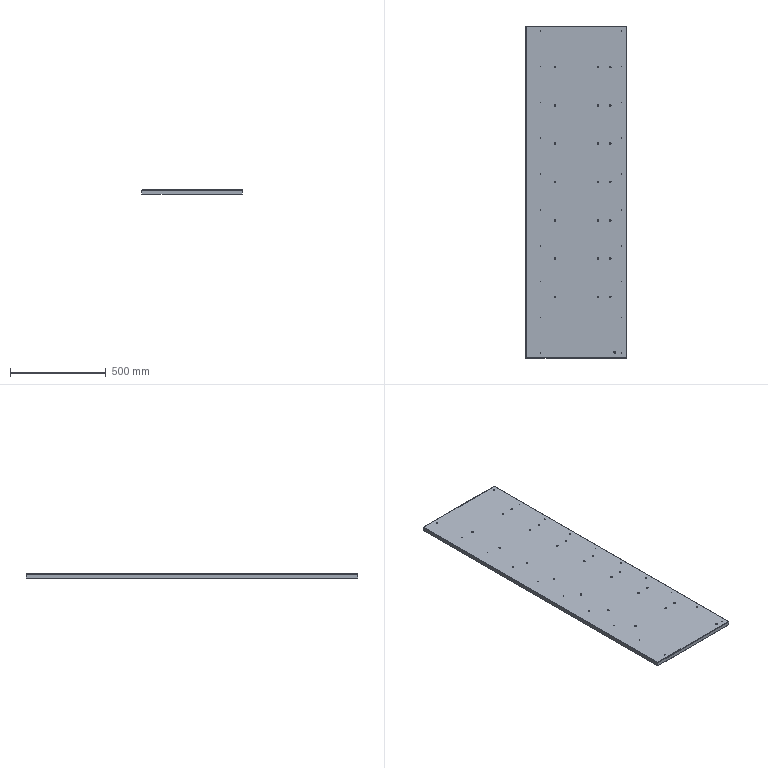Part | SolidWorks | features Cut 2, EdgeFlange 1, FlatPattern 1, ICE 1, SMBaseFlange 1, SheetMetal 1 | 1 solid | 114 faces | box 525 x 1733 x 21 mm | volume 1153064 mm3 | cylinder 90 | plane 20 | spline 4 | commonest cylinder face diameters 8.5 x42 4 x40 2.4 x3 4.8 x3 10 x2